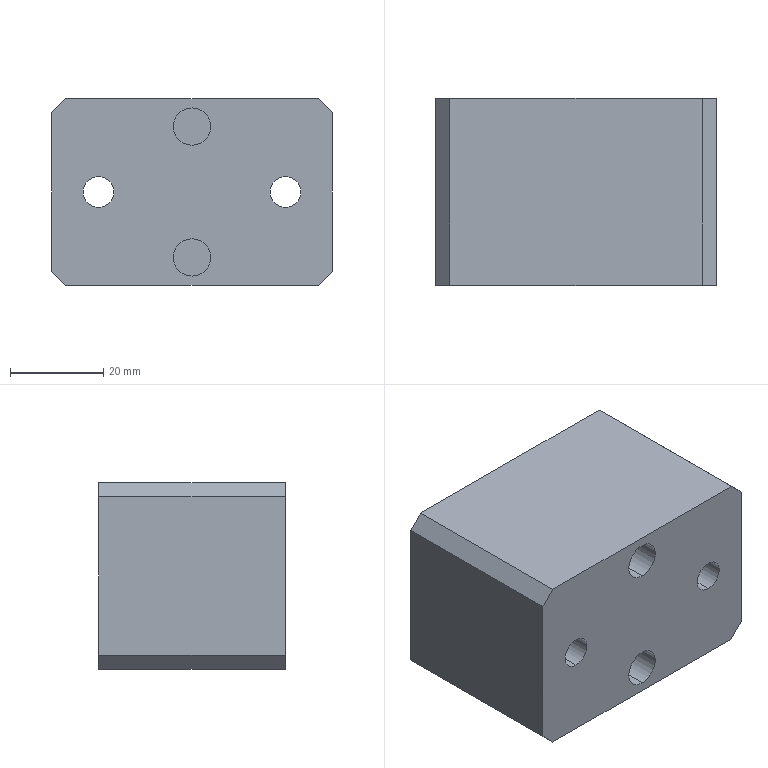Part | SolidWorks | features HoleWzd 4, Chamfer 1, Extrusion 1 | 1 solid | 44 faces | box 60 x 40 x 40 mm | volume 87063 mm3 | cylinder 20 | plane 16 | cone 8 | commonest cylinder face diameters 8 x8 5 x4 6.6 x4 11 x4
STEP:
#1=CARTESIAN_POINT('',(-2.229,-10.711,38.));
#2=VERTEX_POINT('',#1);
#3=CARTESIAN_POINT('',(-2.229,-10.711,30.));
#4=VERTEX_POINT('',#3);
#5=CARTESIAN_POINT('',(-2.229,-10.711,34.));
#6=DIRECTION('',(0.,-1.,0.));
#7=DIRECTION('',(0.,0.,-1.));
#8=AXIS2_PLACEMENT_3D('',#5,#6,#7);
#9=CIRCLE('',#8,4.);
#10=EDGE_CURVE('',#2,#4,#9,.T.);
#11=ORIENTED_EDGE('',*,*,#10,.F.);
#12=CARTESIAN_POINT('',(-2.229,-19.211,38.));
#13=VERTEX_POINT('',#12);
#14=CARTESIAN_POINT('',(-2.229,-19.211,38.));
#15=DIRECTION('',(0.,-1.,0.));
#16=VECTOR('',#15,1000.);
#17=LINE('',#14,#16);
#18=EDGE_CURVE('',#2,#13,#17,.T.);
#19=ORIENTED_EDGE('',*,*,#18,.T.);
#20=CARTESIAN_POINT('',(-2.229,-19.211,30.));
#21=VERTEX_POINT('',#20);
#22=CARTESIAN_POINT('',(-2.229,-19.211,34.));
#23=DIRECTION('',(0.,-1.,0.));
#24=DIRECTION('',(0.,0.,-1.));
#25=AXIS2_PLACEMENT_3D('',#22,#23,#24);
#26=CIRCLE('',#25,4.);
#27=EDGE_CURVE('',#13,#21,#26,.T.);
#28=ORIENTED_EDGE('',*,*,#27,.T.);
#29=CARTESIAN_POINT('',(-2.229,-19.211,30.));
#30=DIRECTION('',(0.,-1.,0.));
#31=VECTOR('',#30,1000.);
#32=LINE('',#29,#31);
#33=EDGE_CURVE('',#4,#21,#32,.T.);
#34=ORIENTED_EDGE('',*,*,#33,.F.);
#35=EDGE_LOOP('',(#11,#19,#28,#34));
#36=FACE_OUTER_BOUND('',#35,.T.);
#37=CARTESIAN_POINT('',(-2.229,-19.211,34.));
#38=DIRECTION('',(0.,-1.,0.));
#39=DIRECTION('',(0.,0.,-1.));
#40=AXIS2_PLACEMENT_3D('',#37,#38,#39);
#41=CYLINDRICAL_SURFACE('',#40,4.);
#42=ADVANCED_FACE('',(#36),#41,.F.);
#43=CARTESIAN_POINT('',(-2.229,-10.711,10.));
#44=VERTEX_POINT('',#43);
#45=CARTESIAN_POINT('',(-2.229,-10.711,2.));
#46=VERTEX_POINT('',#45);
#47=CARTESIAN_POINT('',(-2.229,-10.711,6.));
#48=DIRECTION('',(0.,-1.,0.));
#49=DIRECTION('',(0.,0.,-1.));
#50=AXIS2_PLACEMENT_3D('',#47,#48,#49);
#51=CIRCLE('',#50,4.);
#52=EDGE_CURVE('',#44,#46,#51,.T.);
#53=ORIENTED_EDGE('',*,*,#52,.F.);
#54=CARTESIAN_POINT('',(-2.229,-19.211,10.));
#55=VERTEX_POINT('',#54);
#56=CARTESIAN_POINT('',(-2.229,-19.211,10.));
#57=DIRECTION('',(0.,-1.,0.));
#58=VECTOR('',#57,1000.);
#59=LINE('',#56,#58);
#60=EDGE_CURVE('',#44,#55,#59,.T.);
#61=ORIENTED_EDGE('',*,*,#60,.T.);
#62=CARTESIAN_POINT('',(-2.229,-19.211,2.));
#63=VERTEX_POINT('',#62);
#64=CARTESIAN_POINT('',(-2.229,-19.211,6.));
#65=DIRECTION('',(0.,-1.,0.));
#66=DIRECTION('',(0.,0.,-1.));
#67=AXIS2_PLACEMENT_3D('',#64,#65,#66);
#68=CIRCLE('',#67,4.);
#69=EDGE_CURVE('',#55,#63,#68,.T.);
#70=ORIENTED_EDGE('',*,*,#69,.T.);
#71=CARTESIAN_POINT('',(-2.229,-19.211,2.));
#72=DIRECTION('',(0.,-1.,0.));
#73=VECTOR('',#72,1000.);
#74=LINE('',#71,#73);
#75=EDGE_CURVE('',#46,#63,#74,.T.);
#76=ORIENTED_EDGE('',*,*,#75,.F.);
#77=EDGE_LOOP('',(#53,#61,#70,#76));
#78=FACE_OUTER_BOUND('',#77,.T.);
#79=CARTESIAN_POINT('',(-2.229,-19.211,6.));
#80=DIRECTION('',(0.,-1.,0.));
#81=DIRECTION('',(0.,0.,-1.));
#82=AXIS2_PLACEMENT_3D('',#79,#80,#81);
#83=CYLINDRICAL_SURFACE('',#82,4.);
#84=ADVANCED_FACE('',(#78),#83,.F.);
#85=CARTESIAN_POINT('',(17.771,11.789,4.));
#86=VERTEX_POINT('',#85);
#87=CARTESIAN_POINT('',(17.771,11.789,12.));
#88=VERTEX_POINT('',#87);
#89=CARTESIAN_POINT('',(17.771,11.789,8.));
#90=DIRECTION('',(0.,1.,0.));
#91=DIRECTION('',(0.,0.,1.));
#92=AXIS2_PLACEMENT_3D('',#89,#90,#91);
#93=CIRCLE('',#92,4.);
#94=EDGE_CURVE('',#86,#88,#93,.T.);
#95=ORIENTED_EDGE('',*,*,#94,.F.);
#96=CARTESIAN_POINT('',(17.771,20.789,4.));
#97=VERTEX_POINT('',#96);
#98=CARTESIAN_POINT('',(17.771,20.789,4.));
#99=DIRECTION('',(0.,1.,0.));
#100=VECTOR('',#99,1000.);
#101=LINE('',#98,#100);
#102=EDGE_CURVE('',#86,#97,#101,.T.);
#103=ORIENTED_EDGE('',*,*,#102,.T.);
#104=CARTESIAN_POINT('',(17.771,20.789,12.));
#105=VERTEX_POINT('',#104);
#106=CARTESIAN_POINT('',(17.771,20.789,8.));
#107=DIRECTION('',(0.,1.,0.));
#108=DIRECTION('',(0.,0.,1.));
#109=AXIS2_PLACEMENT_3D('',#106,#107,#108);
#110=CIRCLE('',#109,4.);
#111=EDGE_CURVE('',#97,#105,#110,.T.);
#112=ORIENTED_EDGE('',*,*,#111,.T.);
#113=CARTESIAN_POINT('',(17.771,20.789,12.));
#114=DIRECTION('',(0.,1.,0.));
#115=VECTOR('',#114,1000.);
#116=LINE('',#113,#115);
#117=EDGE_CURVE('',#88,#105,#116,.T.);
#118=ORIENTED_EDGE('',*,*,#117,.F.);
#119=EDGE_LOOP('',(#95,#103,#112,#118));
#120=FACE_OUTER_BOUND('',#119,.T.);
#121=CARTESIAN_POINT('',(17.771,20.789,8.));
#122=DIRECTION('',(0.,1.,0.));
#123=DIRECTION('',(0.,0.,1.));
#124=AXIS2_PLACEMENT_3D('',#121,#122,#123);
#125=CYLINDRICAL_SURFACE('',#124,4.);
#126=ADVANCED_FACE('',(#120),#125,.F.);
#127=CARTESIAN_POINT('',(-22.229,11.789,28.));
#128=VERTEX_POINT('',#127);
#129=CARTESIAN_POINT('',(-22.229,11.789,36.));
#130=VERTEX_POINT('',#129);
#131=CARTESIAN_POINT('',(-22.229,11.789,32.));
#132=DIRECTION('',(0.,1.,0.));
#133=DIRECTION('',(0.,0.,1.));
#134=AXIS2_PLACEMENT_3D('',#131,#132,#133);
#135=CIRCLE('',#134,4.);
#136=EDGE_CURVE('',#128,#130,#135,.T.);
#137=ORIENTED_EDGE('',*,*,#136,.F.);
#138=CARTESIAN_POINT('',(-22.229,20.789,28.));
#139=VERTEX_POINT('',#138);
#140=CARTESIAN_POINT('',(-22.229,20.789,28.));
#141=DIRECTION('',(0.,1.,0.));
#142=VECTOR('',#141,1000.);
#143=LINE('',#140,#142);
#144=EDGE_CURVE('',#128,#139,#143,.T.);
#145=ORIENTED_EDGE('',*,*,#144,.T.);
#146=CARTESIAN_POINT('',(-22.229,20.789,36.));
#147=VERTEX_POINT('',#146);
#148=CARTESIAN_POINT('',(-22.229,20.789,32.));
#149=DIRECTION('',(0.,1.,0.));
#150=DIRECTION('',(0.,0.,1.));
#151=AXIS2_PLACEMENT_3D('',#148,#149,#150);
#152=CIRCLE('',#151,4.);
#153=EDGE_CURVE('',#139,#147,#152,.T.);
#154=ORIENTED_EDGE('',*,*,#153,.T.);
#155=CARTESIAN_POINT('',(-22.229,20.789,36.));
#156=DIRECTION('',(0.,1.,0.));
#157=VECTOR('',#156,1000.);
#158=LINE('',#155,#157);
#159=EDGE_CURVE('',#130,#147,#158,.T.);
#160=ORIENTED_EDGE('',*,*,#159,.F.);
#161=EDGE_LOOP('',(#137,#145,#154,#160));
#162=FACE_OUTER_BOUND('',#161,.T.);
#163=CARTESIAN_POINT('',(-22.229,20.789,32.));
#164=DIRECTION('',(0.,1.,0.));
#165=DIRECTION('',(0.,0.,1.));
#166=AXIS2_PLACEMENT_3D('',#163,#164,#165);
#167=CYLINDRICAL_SURFACE('',#166,4.);
#168=ADVANCED_FACE('',(#162),#167,.F.);
#169=CARTESIAN_POINT('',(-22.229,-6.211,14.5));
#170=VERTEX_POINT('',#169);
#171=CARTESIAN_POINT('',(-22.229,-6.211,25.5));
#172=VERTEX_POINT('',#171);
#173=CARTESIAN_POINT('',(-22.229,-6.211,20.));
#174=DIRECTION('',(0.,1.,0.));
#175=DIRECTION('',(0.,0.,1.));
#176=AXIS2_PLACEMENT_3D('',#173,#174,#175);
#177=CIRCLE('',#176,5.5);
#178=EDGE_CURVE('',#170,#172,#177,.T.);
#179=ORIENTED_EDGE('',*,*,#178,.F.);
#180=CARTESIAN_POINT('',(-22.229,20.789,14.5));
#181=VERTEX_POINT('',#180);
#182=CARTESIAN_POINT('',(-22.229,20.789,14.5));
#183=DIRECTION('',(0.,1.,0.));
#184=VECTOR('',#183,1000.);
#185=LINE('',#182,#184);
#186=EDGE_CURVE('',#170,#181,#185,.T.);
#187=ORIENTED_EDGE('',*,*,#186,.T.);
#188=CARTESIAN_POINT('',(-22.229,20.789,25.5));
#189=VERTEX_POINT('',#188);
#190=CARTESIAN_POINT('',(-22.229,20.789,20.));
#191=DIRECTION('',(0.,1.,0.));
#192=DIRECTION('',(0.,0.,1.));
#193=AXIS2_PLACEMENT_3D('',#190,#191,#192);
#194=CIRCLE('',#193,5.5);
#195=EDGE_CURVE('',#181,#189,#194,.T.);
#196=ORIENTED_EDGE('',*,*,#195,.T.);
#197=CARTESIAN_POINT('',(-22.229,20.789,25.5));
#198=DIRECTION('',(0.,1.,0.));
#199=VECTOR('',#198,1000.);
#200=LINE('',#197,#199);
#201=EDGE_CURVE('',#172,#189,#200,.T.);
#202=ORIENTED_EDGE('',*,*,#201,.F.);
#203=EDGE_LOOP('',(#179,#187,#196,#202));
#204=FACE_OUTER_BOUND('',#203,.T.);
#205=CARTESIAN_POINT('',(-22.229,20.789,20.));
#206=DIRECTION('',(0.,1.,0.));
#207=DIRECTION('',(0.,0.,1.));
#208=AXIS2_PLACEMENT_3D('',#205,#206,#207);
#209=CYLINDRICAL_SURFACE('',#208,5.5);
#210=ADVANCED_FACE('',(#204),#209,.F.);
#211=CARTESIAN_POINT('',(-22.229,-19.211,16.7));
#212=VERTEX_POINT('',#211);
#213=CARTESIAN_POINT('',(-22.229,-19.211,23.3));
#214=VERTEX_POINT('',#213);
#215=CARTESIAN_POINT('',(-22.229,-19.211,20.));
#216=DIRECTION('',(0.,1.,0.));
#217=DIRECTION('',(0.,0.,1.));
#218=AXIS2_PLACEMENT_3D('',#215,#216,#217);
#219=CIRCLE('',#218,3.3);
#220=EDGE_CURVE('',#212,#214,#219,.T.);
#221=ORIENTED_EDGE('',*,*,#220,.F.);
#222=CARTESIAN_POINT('',(-22.229,-6.211,16.7));
#223=VERTEX_POINT('',#222);
#224=CARTESIAN_POINT('',(-22.229,20.789,16.7));
#225=DIRECTION('',(0.,1.,0.));
#226=VECTOR('',#225,1000.);
#227=LINE('',#224,#226);
#228=EDGE_CURVE('',#212,#223,#227,.T.);
#229=ORIENTED_EDGE('',*,*,#228,.T.);
#230=CARTESIAN_POINT('',(-22.229,-6.211,23.3));
#231=VERTEX_POINT('',#230);
#232=CARTESIAN_POINT('',(-22.229,-6.211,20.));
#233=DIRECTION('',(0.,1.,0.));
#234=DIRECTION('',(0.,0.,1.));
#235=AXIS2_PLACEMENT_3D('',#232,#233,#234);
#236=CIRCLE('',#235,3.3);
#237=EDGE_CURVE('',#223,#231,#236,.T.);
#238=ORIENTED_EDGE('',*,*,#237,.T.);
#239=CARTESIAN_POINT('',(-22.229,20.789,23.3));
#240=DIRECTION('',(0.,1.,0.));
#241=VECTOR('',#240,1000.);
#242=LINE('',#239,#241);
#243=EDGE_CURVE('',#214,#231,#242,.T.);
#244=ORIENTED_EDGE('',*,*,#243,.F.);
#245=EDGE_LOOP('',(#221,#229,#238,#244));
#246=FACE_OUTER_BOUND('',#245,.T.);
#247=CARTESIAN_POINT('',(-22.229,20.789,20.));
#248=DIRECTION('',(0.,1.,0.));
#249=DIRECTION('',(0.,0.,1.));
#250=AXIS2_PLACEMENT_3D('',#247,#248,#249);
#251=CYLINDRICAL_SURFACE('',#250,3.3);
#252=ADVANCED_FACE('',(#246),#251,.F.);
#253=CARTESIAN_POINT('',(17.771,-6.211,14.5));
#254=VERTEX_POINT('',#253);
#255=CARTESIAN_POINT('',(17.771,-6.211,25.5));
#256=VERTEX_POINT('',#255);
#257=CARTESIAN_POINT('',(17.771,-6.211,20.));
#258=DIRECTION('',(0.,1.,0.));
#259=DIRECTION('',(0.,0.,1.));
#260=AXIS2_PLACEMENT_3D('',#257,#258,#259);
#261=CIRCLE('',#260,5.5);
#262=EDGE_CURVE('',#254,#256,#261,.T.);
#263=ORIENTED_EDGE('',*,*,#262,.F.);
#264=CARTESIAN_POINT('',(17.771,20.789,14.5));
#265=VERTEX_POINT('',#264);
#266=CARTESIAN_POINT('',(17.771,20.789,14.5));
#267=DIRECTION('',(0.,1.,0.));
#268=VECTOR('',#267,1000.);
#269=LINE('',#266,#268);
#270=EDGE_CURVE('',#254,#265,#269,.T.);
#271=ORIENTED_EDGE('',*,*,#270,.T.);
#272=CARTESIAN_POINT('',(17.771,20.789,25.5));
#273=VERTEX_POINT('',#272);
#274=CARTESIAN_POINT('',(17.771,20.789,20.));
#275=DIRECTION('',(0.,1.,0.));
#276=DIRECTION('',(0.,0.,1.));
#277=AXIS2_PLACEMENT_3D('',#274,#275,#276);
#278=CIRCLE('',#277,5.5);
#279=EDGE_CURVE('',#265,#273,#278,.T.);
#280=ORIENTED_EDGE('',*,*,#279,.T.);
#281=CARTESIAN_POINT('',(17.771,20.789,25.5));
#282=DIRECTION('',(0.,1.,0.));
#283=VECTOR('',#282,1000.);
#284=LINE('',#281,#283);
#285=EDGE_CURVE('',#256,#273,#284,.T.);
#286=ORIENTED_EDGE('',*,*,#285,.F.);
#287=EDGE_LOOP('',(#263,#271,#280,#286));
#288=FACE_OUTER_BOUND('',#287,.T.);
#289=CARTESIAN_POINT('',(17.771,20.789,20.));
#290=DIRECTION('',(0.,1.,0.));
#291=DIRECTION('',(0.,0.,1.));
#292=AXIS2_PLACEMENT_3D('',#289,#290,#291);
#293=CYLINDRICAL_SURFACE('',#292,5.5);
#294=ADVANCED_FACE('',(#288),#293,.F.);
#295=CARTESIAN_POINT('',(17.771,-19.211,16.7));
#296=VERTEX_POINT('',#295);
#297=CARTESIAN_POINT('',(17.771,-19.211,23.3));
#298=VERTEX_POINT('',#297);
#299=CARTESIAN_POINT('',(17.771,-19.211,20.));
#300=DIRECTION('',(0.,1.,0.));
#301=DIRECTION('',(0.,0.,1.));
#302=AXIS2_PLACEMENT_3D('',#299,#300,#301);
#303=CIRCLE('',#302,3.3);
#304=EDGE_CURVE('',#296,#298,#303,.T.);
#305=ORIENTED_EDGE('',*,*,#304,.F.);
#306=CARTESIAN_POINT('',(17.771,-6.211,16.7));
#307=VERTEX_POINT('',#306);
#308=CARTESIAN_POINT('',(17.771,20.789,16.7));
#309=DIRECTION('',(0.,1.,0.));
#310=VECTOR('',#309,1000.);
#311=LINE('',#308,#310);
#312=EDGE_CURVE('',#296,#307,#311,.T.);
#313=ORIENTED_EDGE('',*,*,#312,.T.);
#314=CARTESIAN_POINT('',(17.771,-6.211,23.3));
#315=VERTEX_POINT('',#314);
#316=CARTESIAN_POINT('',(17.771,-6.211,20.));
#317=DIRECTION('',(0.,1.,0.));
#318=DIRECTION('',(0.,0.,1.));
#319=AXIS2_PLACEMENT_3D('',#316,#317,#318);
#320=CIRCLE('',#319,3.3);
#321=EDGE_CURVE('',#307,#315,#320,.T.);
#322=ORIENTED_EDGE('',*,*,#321,.T.);
#323=CARTESIAN_POINT('',(17.771,20.789,23.3));
#324=DIRECTION('',(0.,1.,0.));
#325=VECTOR('',#324,1000.);
#326=LINE('',#323,#325);
#327=EDGE_CURVE('',#298,#315,#326,.T.);
#328=ORIENTED_EDGE('',*,*,#327,.F.);
#329=EDGE_LOOP('',(#305,#313,#322,#328));
#330=FACE_OUTER_BOUND('',#329,.T.);
#331=CARTESIAN_POINT('',(17.771,20.789,20.));
#332=DIRECTION('',(0.,1.,0.));
#333=DIRECTION('',(0.,0.,1.));
#334=AXIS2_PLACEMENT_3D('',#331,#332,#333);
#335=CYLINDRICAL_SURFACE('',#334,3.3);
#336=ADVANCED_FACE('',(#330),#335,.F.);
#337=CARTESIAN_POINT('',(-22.229,20.264,5.5));
#338=VERTEX_POINT('',#337);
#339=CARTESIAN_POINT('',(-22.229,20.264,10.5));
#340=VERTEX_POINT('',#339);
#341=CARTESIAN_POINT('',(-22.229,20.264,8.));
#342=DIRECTION('',(0.,1.,0.));
#343=DIRECTION('',(0.,0.,1.));
#344=AXIS2_PLACEMENT_3D('',#341,#342,#343);
#345=CIRCLE('',#344,2.5);
#346=EDGE_CURVE('',#338,#340,#345,.T.);
#347=ORIENTED_EDGE('',*,*,#346,.F.);
#348=CARTESIAN_POINT('',(-22.229,20.789,4.975));
#349=VERTEX_POINT('',#348);
#350=CARTESIAN_POINT('',(-22.229,20.789,4.975));
#351=DIRECTION('',(0.,0.7071,-0.7071));
#352=VECTOR('',#351,1000.);
#353=LINE('',#350,#352);
#354=EDGE_CURVE('',#338,#349,#353,.T.);
#355=ORIENTED_EDGE('',*,*,#354,.T.);
#356=CARTESIAN_POINT('',(-22.229,20.789,11.025));
#357=VERTEX_POINT('',#356);
#358=CARTESIAN_POINT('',(-22.229,20.789,8.));
#359=DIRECTION('',(0.,1.,0.));
#360=DIRECTION('',(0.,0.,1.));
#361=AXIS2_PLACEMENT_3D('',#358,#359,#360);
#362=CIRCLE('',#361,3.025);
#363=EDGE_CURVE('',#349,#357,#362,.T.);
#364=ORIENTED_EDGE('',*,*,#363,.T.);
#365=CARTESIAN_POINT('',(-22.229,20.789,11.025));
#366=DIRECTION('',(0.,0.7071,0.7071));
#367=VECTOR('',#366,1000.);
#368=LINE('',#365,#367);
#369=EDGE_CURVE('',#340,#357,#368,.T.);
#370=ORIENTED_EDGE('',*,*,#369,.F.);
#371=EDGE_LOOP('',(#347,#355,#364,#370));
#372=FACE_OUTER_BOUND('',#371,.T.);
#373=CARTESIAN_POINT('',(-22.229,20.789,8.));
#374=DIRECTION('',(0.,1.,0.));
#375=DIRECTION('',(0.,0.,1.));
#376=AXIS2_PLACEMENT_3D('',#373,#374,#375);
#377=CONICAL_SURFACE('',#376,3.025,0.7854);
#378=ADVANCED_FACE('',(#372),#377,.F.);
#379=CARTESIAN_POINT('',(-22.229,10.292,5.5));
#380=VERTEX_POINT('',#379);
#381=CARTESIAN_POINT('',(-22.229,10.292,10.5));
#382=VERTEX_POINT('',#381);
#383=CARTESIAN_POINT('',(-22.229,10.292,8.));
#384=DIRECTION('',(0.,1.,0.));
#385=DIRECTION('',(0.,0.,1.));
#386=AXIS2_PLACEMENT_3D('',#383,#384,#385);
#387=CIRCLE('',#386,2.5);
#388=EDGE_CURVE('',#380,#382,#387,.T.);
#389=ORIENTED_EDGE('',*,*,#388,.F.);
#390=CARTESIAN_POINT('',(-22.229,20.789,5.5));
#391=DIRECTION('',(0.,1.,0.));
#392=VECTOR('',#391,1000.);
#393=LINE('',#390,#392);
#394=EDGE_CURVE('',#380,#338,#393,.T.);
#395=ORIENTED_EDGE('',*,*,#394,.T.);
#396=ORIENTED_EDGE('',*,*,#346,.T.);
#397=CARTESIAN_POINT('',(-22.229,20.789,10.5));
#398=DIRECTION('',(0.,1.,0.));
#399=VECTOR('',#398,1000.);
#400=LINE('',#397,#399);
#401=EDGE_CURVE('',#382,#340,#400,.T.);
#402=ORIENTED_EDGE('',*,*,#401,.F.);
#403=EDGE_LOOP('',(#389,#395,#396,#402));
#404=FACE_OUTER_BOUND('',#403,.T.);
#405=CARTESIAN_POINT('',(-22.229,20.789,8.));
#406=DIRECTION('',(0.,1.,0.));
#407=DIRECTION('',(0.,0.,1.));
#408=AXIS2_PLACEMENT_3D('',#405,#406,#407);
#409=CYLINDRICAL_SURFACE('',#408,2.5);
#410=ADVANCED_FACE('',(#404),#409,.F.);
#411=CARTESIAN_POINT('',(-22.229,8.789,8.));
#412=VERTEX_POINT('',#411);
#413=CARTESIAN_POINT('',(-22.229,10.292,10.5));
#414=DIRECTION('',(0.,0.515,0.8572));
#415=VECTOR('',#414,1000.);
#416=LINE('',#413,#415);
#417=EDGE_CURVE('',#412,#382,#416,.T.);
#418=ORIENTED_EDGE('',*,*,#417,.F.);
#419=CARTESIAN_POINT('',(-22.229,10.292,5.5));
#420=DIRECTION('',(0.,0.515,-0.8572));
#421=VECTOR('',#420,1000.);
#422=LINE('',#419,#421);
#423=EDGE_CURVE('',#412,#380,#422,.T.);
#424=ORIENTED_EDGE('',*,*,#423,.T.);
#425=ORIENTED_EDGE('',*,*,#388,.T.);
#426=EDGE_LOOP('',(#418,#424,#425));
#427=FACE_OUTER_BOUND('',#426,.T.);
#428=CARTESIAN_POINT('',(-22.229,10.292,8.));
#429=DIRECTION('',(0.,1.,0.));
#430=DIRECTION('',(0.,0.,1.));
#431=AXIS2_PLACEMENT_3D('',#428,#429,#430);
#432=CONICAL_SURFACE('',#431,2.5,1.03);
#433=ADVANCED_FACE('',(#427),#432,.F.);
#434=CARTESIAN_POINT('',(17.771,20.264,29.5));
#435=VERTEX_POINT('',#434);
#436=CARTESIAN_POINT('',(17.771,20.264,34.5));
#437=VERTEX_POINT('',#436);
#438=CARTESIAN_POINT('',(17.771,20.264,32.));
#439=DIRECTION('',(0.,1.,0.));
#440=DIRECTION('',(0.,0.,1.));
#441=AXIS2_PLACEMENT_3D('',#438,#439,#440);
#442=CIRCLE('',#441,2.5);
#443=EDGE_CURVE('',#435,#437,#442,.T.);
#444=ORIENTED_EDGE('',*,*,#443,.F.);
#445=CARTESIAN_POINT('',(17.771,20.789,28.975));
#446=VERTEX_POINT('',#445);
#447=CARTESIAN_POINT('',(17.771,20.789,28.975));
#448=DIRECTION('',(0.,0.7071,-0.7071));
#449=VECTOR('',#448,1000.);
#450=LINE('',#447,#449);
#451=EDGE_CURVE('',#435,#446,#450,.T.);
#452=ORIENTED_EDGE('',*,*,#451,.T.);
#453=CARTESIAN_POINT('',(17.771,20.789,35.025));
#454=VERTEX_POINT('',#453);
#455=CARTESIAN_POINT('',(17.771,20.789,32.));
#456=DIRECTION('',(0.,1.,0.));
#457=DIRECTION('',(0.,0.,1.));
#458=AXIS2_PLACEMENT_3D('',#455,#456,#457);
#459=CIRCLE('',#458,3.025);
#460=EDGE_CURVE('',#446,#454,#459,.T.);
#461=ORIENTED_EDGE('',*,*,#460,.T.);
#462=CARTESIAN_POINT('',(17.771,20.789,35.025));
#463=DIRECTION('',(0.,0.7071,0.7071));
#464=VECTOR('',#463,1000.);
#465=LINE('',#462,#464);
#466=EDGE_CURVE('',#437,#454,#465,.T.);
#467=ORIENTED_EDGE('',*,*,#466,.F.);
#468=EDGE_LOOP('',(#444,#452,#461,#467));
#469=FACE_OUTER_BOUND('',#468,.T.);
#470=CARTESIAN_POINT('',(17.771,20.789,32.));
#471=DIRECTION('',(0.,1.,0.));
#472=DIRECTION('',(0.,0.,1.));
#473=AXIS2_PLACEMENT_3D('',#470,#471,#472);
#474=CONICAL_SURFACE('',#473,3.025,0.7854);
#475=ADVANCED_FACE('',(#469),#474,.F.);
#476=CARTESIAN_POINT('',(17.771,10.292,29.5));
#477=VERTEX_POINT('',#476);
#478=CARTESIAN_POINT('',(17.771,10.292,34.5));
#479=VERTEX_POINT('',#478);
#480=CARTESIAN_POINT('',(17.771,10.292,32.));
#481=DIRECTION('',(0.,1.,0.));
#482=DIRECTION('',(0.,0.,1.));
#483=AXIS2_PLACEMENT_3D('',#480,#481,#482);
#484=CIRCLE('',#483,2.5);
#485=EDGE_CURVE('',#477,#479,#484,.T.);
#486=ORIENTED_EDGE('',*,*,#485,.F.);
#487=CARTESIAN_POINT('',(17.771,20.789,29.5));
#488=DIRECTION('',(0.,1.,0.));
#489=VECTOR('',#488,1000.);
#490=LINE('',#487,#489);
#491=EDGE_CURVE('',#477,#435,#490,.T.);
#492=ORIENTED_EDGE('',*,*,#491,.T.);
#493=ORIENTED_EDGE('',*,*,#443,.T.);
#494=CARTESIAN_POINT('',(17.771,20.789,34.5));
#495=DIRECTION('',(0.,1.,0.));
#496=VECTOR('',#495,1000.);
#497=LINE('',#494,#496);
#498=EDGE_CURVE('',#479,#437,#497,.T.);
#499=ORIENTED_EDGE('',*,*,#498,.F.);
#500=EDGE_LOOP('',(#486,#492,#493,#499));
#501=FACE_OUTER_BOUND('',#500,.T.);
#502=CARTESIAN_POINT('',(17.771,20.789,32.));
#503=DIRECTION('',(0.,1.,0.));
#504=DIRECTION('',(0.,0.,1.));
#505=AXIS2_PLACEMENT_3D('',#502,#503,#504);
#506=CYLINDRICAL_SURFACE('',#505,2.5);
#507=ADVANCED_FACE('',(#501),#506,.F.);
#508=CARTESIAN_POINT('',(17.771,8.789,32.));
#509=VERTEX_POINT('',#508);
#510=CARTESIAN_POINT('',(17.771,10.292,34.5));
#511=DIRECTION('',(0.,0.515,0.8572));
#512=VECTOR('',#511,1000.);
#513=LINE('',#510,#512);
#514=EDGE_CURVE('',#509,#479,#513,.T.);
#515=ORIENTED_EDGE('',*,*,#514,.F.);
#516=CARTESIAN_POINT('',(17.771,10.292,29.5));
#517=DIRECTION('',(0.,0.515,-0.8572));
#518=VECTOR('',#517,1000.);
#519=LINE('',#516,#518);
#520=EDGE_CURVE('',#509,#477,#519,.T.);
#521=ORIENTED_EDGE('',*,*,#520,.T.);
#522=ORIENTED_EDGE('',*,*,#485,.T.);
#523=EDGE_LOOP('',(#515,#521,#522));
#524=FACE_OUTER_BOUND('',#523,.T.);
#525=CARTESIAN_POINT('',(17.771,10.292,32.));
#526=DIRECTION('',(0.,1.,0.));
#527=DIRECTION('',(0.,0.,1.));
#528=AXIS2_PLACEMENT_3D('',#525,#526,#527);
#529=CONICAL_SURFACE('',#528,2.5,1.03);
#530=ADVANCED_FACE('',(#524),#529,.F.);
#531=CARTESIAN_POINT('',(-32.229,-19.211,37.));
#532=VERTEX_POINT('',#531);
#533=CARTESIAN_POINT('',(-32.229,-19.211,3.));
#534=VERTEX_POINT('',#533);
#535=CARTESIAN_POINT('',(-32.229,-19.211,40.));
#536=DIRECTION('',(0.,0.,-1.));
#537=VECTOR('',#536,1000.);
#538=LINE('',#535,#537);
#539=EDGE_CURVE('',#532,#534,#538,.T.);
#540=ORIENTED_EDGE('',*,*,#539,.F.);
#541=CARTESIAN_POINT('',(-32.229,20.789,37.));
#542=VERTEX_POINT('',#541);
#543=CARTESIAN_POINT('',(-32.229,20.789,37.));
#544=DIRECTION('',(0.,1.,0.));
#545=VECTOR('',#544,1000.);
#546=LINE('',#543,#545);
#547=EDGE_CURVE('',#532,#542,#546,.T.);
#548=ORIENTED_EDGE('',*,*,#547,.T.);
#549=CARTESIAN_POINT('',(-32.229,20.789,3.));
#550=VERTEX_POINT('',#549);
#551=CARTESIAN_POINT('',(-32.229,20.789,40.));
#552=DIRECTION('',(0.,0.,-1.));
#553=VECTOR('',#552,1000.);
#554=LINE('',#551,#553);
#555=EDGE_CURVE('',#542,#550,#554,.T.);
#556=ORIENTED_EDGE('',*,*,#555,.T.);
#557=CARTESIAN_POINT('',(-32.229,20.789,3.));
#558=DIRECTION('',(0.,-1.,0.));
#559=VECTOR('',#558,1000.);
#560=LINE('',#557,#559);
#561=EDGE_CURVE('',#550,#534,#560,.T.);
#562=ORIENTED_EDGE('',*,*,#561,.T.);
#563=EDGE_LOOP('',(#540,#548,#556,#562));
#564=FACE_OUTER_BOUND('',#563,.T.);
#565=CARTESIAN_POINT('',(-32.229,20.789,40.));
#566=DIRECTION('',(1.,0.,0.));
#567=DIRECTION('',(0.,1.,0.));
#568=AXIS2_PLACEMENT_3D('',#565,#566,#567);
#569=PLANE('',#568);
#570=ADVANCED_FACE('',(#564),#569,.F.);
#571=CARTESIAN_POINT('',(-2.229,-19.211,34.));
#572=DIRECTION('',(0.,-1.,0.));
#573=DIRECTION('',(0.,0.,-1.));
#574=AXIS2_PLACEMENT_3D('',#571,#572,#573);
#575=CIRCLE('',#574,4.);
#576=EDGE_CURVE('',#21,#13,#575,.T.);
#577=ORIENTED_EDGE('',*,*,#576,.F.);
#578=ORIENTED_EDGE('',*,*,#27,.F.);
#579=EDGE_LOOP('',(#577,#578));
#580=FACE_BOUND('',#579,.T.);
#581=CARTESIAN_POINT('',(-2.229,-19.211,6.));
#582=DIRECTION('',(0.,-1.,0.));
#583=DIRECTION('',(0.,0.,-1.));
#584=AXIS2_PLACEMENT_3D('',#581,#582,#583);
#585=CIRCLE('',#584,4.);
#586=EDGE_CURVE('',#63,#55,#585,.T.);
#587=ORIENTED_EDGE('',*,*,#586,.F.);
#588=ORIENTED_EDGE('',*,*,#69,.F.);
#589=EDGE_LOOP('',(#587,#588));
#590=FACE_BOUND('',#589,.T.);
#591=CARTESIAN_POINT('',(-22.229,-19.211,20.));
#592=DIRECTION('',(0.,1.,0.));
#593=DIRECTION('',(0.,0.,1.));
#594=AXIS2_PLACEMENT_3D('',#591,#592,#593);
#595=CIRCLE('',#594,3.3);
#596=EDGE_CURVE('',#214,#212,#595,.T.);
#597=ORIENTED_EDGE('',*,*,#596,.T.);
#598=ORIENTED_EDGE('',*,*,#220,.T.);
#599=EDGE_LOOP('',(#597,#598));
#600=FACE_BOUND('',#599,.T.);
#601=CARTESIAN_POINT('',(17.771,-19.211,20.));
#602=DIRECTION('',(0.,1.,0.));
#603=DIRECTION('',(0.,0.,1.));
#604=AXIS2_PLACEMENT_3D('',#601,#602,#603);
#605=CIRCLE('',#604,3.3);
#606=EDGE_CURVE('',#298,#296,#605,.T.);
#607=ORIENTED_EDGE('',*,*,#606,.T.);
#608=ORIENTED_EDGE('',*,*,#304,.T.);
#609=EDGE_LOOP('',(#607,#608));
#610=FACE_BOUND('',#609,.T.);
#611=CARTESIAN_POINT('',(27.771,-19.211,37.));
#612=VERTEX_POINT('',#611);
#613=CARTESIAN_POINT('',(27.771,-19.211,3.));
#614=VERTEX_POINT('',#613);
#615=CARTESIAN_POINT('',(27.771,-19.211,40.));
#616=DIRECTION('',(0.,0.,-1.));
#617=VECTOR('',#616,1000.);
#618=LINE('',#615,#617);
#619=EDGE_CURVE('',#612,#614,#618,.T.);
#620=ORIENTED_EDGE('',*,*,#619,.F.);
#621=CARTESIAN_POINT('',(24.771,-19.211,40.));
#622=VERTEX_POINT('',#621);
#623=CARTESIAN_POINT('',(24.771,-19.211,40.));
#624=DIRECTION('',(-0.7071,0.,0.7071));
#625=VECTOR('',#624,1000.);
#626=LINE('',#623,#625);
#627=EDGE_CURVE('',#612,#622,#626,.T.);
#628=ORIENTED_EDGE('',*,*,#627,.T.);
#629=CARTESIAN_POINT('',(-29.229,-19.211,40.));
#630=VERTEX_POINT('',#629);
#631=CARTESIAN_POINT('',(-32.229,-19.211,40.));
#632=DIRECTION('',(1.,0.,0.));
#633=VECTOR('',#632,1000.);
#634=LINE('',#631,#633);
#635=EDGE_CURVE('',#630,#622,#634,.T.);
#636=ORIENTED_EDGE('',*,*,#635,.F.);
#637=CARTESIAN_POINT('',(-29.229,-19.211,40.));
#638=DIRECTION('',(-0.7071,0.,-0.7071));
#639=VECTOR('',#638,1000.);
#640=LINE('',#637,#639);
#641=EDGE_CURVE('',#630,#532,#640,.T.);
#642=ORIENTED_EDGE('',*,*,#641,.T.);
#643=ORIENTED_EDGE('',*,*,#539,.T.);
#644=CARTESIAN_POINT('',(-29.229,-19.211,0.));
#645=VERTEX_POINT('',#644);
#646=CARTESIAN_POINT('',(-32.229,-19.211,3.));
#647=DIRECTION('',(0.7071,0.,-0.7071));
#648=VECTOR('',#647,1000.);
#649=LINE('',#646,#648);
#650=EDGE_CURVE('',#534,#645,#649,.T.);
#651=ORIENTED_EDGE('',*,*,#650,.T.);
#652=CARTESIAN_POINT('',(24.771,-19.211,0.));
#653=VERTEX_POINT('',#652);
#654=CARTESIAN_POINT('',(-32.229,-19.211,0.));
#655=DIRECTION('',(1.,0.,0.));
#656=VECTOR('',#655,1000.);
#657=LINE('',#654,#656);
#658=EDGE_CURVE('',#645,#653,#657,.T.);
#659=ORIENTED_EDGE('',*,*,#658,.T.);
#660=CARTESIAN_POINT('',(27.771,-19.211,3.));
#661=DIRECTION('',(0.7071,0.,0.7071));
#662=VECTOR('',#661,1000.);
#663=LINE('',#660,#662);
#664=EDGE_CURVE('',#653,#614,#663,.T.);
#665=ORIENTED_EDGE('',*,*,#664,.T.);
#666=EDGE_LOOP('',(#620,#628,#636,#642,#643,#651,#659,#665));
#667=FACE_OUTER_BOUND('',#666,.T.);
#668=CARTESIAN_POINT('',(-32.229,-19.211,40.));
#669=DIRECTION('',(0.,1.,0.));
#670=DIRECTION('',(0.,0.,1.));
#671=AXIS2_PLACEMENT_3D('',#668,#669,#670);
#672=PLANE('',#671);
#673=ADVANCED_FACE('',(#580,#590,#600,#610,#667),#672,.F.);
#674=CARTESIAN_POINT('',(27.771,20.789,37.));
#675=VERTEX_POINT('',#674);
#676=CARTESIAN_POINT('',(27.771,20.789,3.));
#677=VERTEX_POINT('',#676);
#678=CARTESIAN_POINT('',(27.771,20.789,40.));
#679=DIRECTION('',(0.,0.,-1.));
#680=VECTOR('',#679,1000.);
#681=LINE('',#678,#680);
#682=EDGE_CURVE('',#675,#677,#681,.T.);
#683=ORIENTED_EDGE('',*,*,#682,.F.);
#684=CARTESIAN_POINT('',(27.771,-19.211,37.));
#685=DIRECTION('',(0.,-1.,0.));
#686=VECTOR('',#685,1000.);
#687=LINE('',#684,#686);
#688=EDGE_CURVE('',#675,#612,#687,.T.);
#689=ORIENTED_EDGE('',*,*,#688,.T.);
#690=ORIENTED_EDGE('',*,*,#619,.T.);
#691=CARTESIAN_POINT('',(27.771,20.789,3.));
#692=DIRECTION('',(0.,1.,0.));
#693=VECTOR('',#692,1000.);
#694=LINE('',#691,#693);
#695=EDGE_CURVE('',#614,#677,#694,.T.);
#696=ORIENTED_EDGE('',*,*,#695,.T.);
#697=EDGE_LOOP('',(#683,#689,#690,#696));
#698=FACE_OUTER_BOUND('',#697,.T.);
#699=CARTESIAN_POINT('',(27.771,20.789,40.));
#700=DIRECTION('',(-1.,0.,0.));
#701=DIRECTION('',(0.,-1.,0.));
#702=AXIS2_PLACEMENT_3D('',#699,#700,#701);
#703=PLANE('',#702);
#704=ADVANCED_FACE('',(#698),#703,.F.);
#705=CARTESIAN_POINT('',(17.771,20.789,8.));
#706=DIRECTION('',(0.,1.,0.));
#707=DIRECTION('',(0.,0.,1.));
#708=AXIS2_PLACEMENT_3D('',#705,#706,#707);
#709=CIRCLE('',#708,4.);
#710=EDGE_CURVE('',#105,#97,#709,.T.);
#711=ORIENTED_EDGE('',*,*,#710,.F.);
#712=ORIENTED_EDGE('',*,*,#111,.F.);
#713=EDGE_LOOP('',(#711,#712));
#714=FACE_BOUND('',#713,.T.);
#715=CARTESIAN_POINT('',(-22.229,20.789,32.));
#716=DIRECTION('',(0.,1.,0.));
#717=DIRECTION('',(0.,0.,1.));
#718=AXIS2_PLACEMENT_3D('',#715,#716,#717);
#719=CIRCLE('',#718,4.);
#720=EDGE_CURVE('',#147,#139,#719,.T.);
#721=ORIENTED_EDGE('',*,*,#720,.F.);
#722=ORIENTED_EDGE('',*,*,#153,.F.);
#723=EDGE_LOOP('',(#721,#722));
#724=FACE_BOUND('',#723,.T.);
#725=CARTESIAN_POINT('',(-22.229,20.789,20.));
#726=DIRECTION('',(0.,1.,0.));
#727=DIRECTION('',(0.,0.,1.));
#728=AXIS2_PLACEMENT_3D('',#725,#726,#727);
#729=CIRCLE('',#728,5.5);
#730=EDGE_CURVE('',#189,#181,#729,.T.);
#731=ORIENTED_EDGE('',*,*,#730,.F.);
#732=ORIENTED_EDGE('',*,*,#195,.F.);
#733=EDGE_LOOP('',(#731,#732));
#734=FACE_BOUND('',#733,.T.);
#735=CARTESIAN_POINT('',(17.771,20.789,20.));
#736=DIRECTION('',(0.,1.,0.));
#737=DIRECTION('',(0.,0.,1.));
#738=AXIS2_PLACEMENT_3D('',#735,#736,#737);
#739=CIRCLE('',#738,5.5);
#740=EDGE_CURVE('',#273,#265,#739,.T.);
#741=ORIENTED_EDGE('',*,*,#740,.F.);
#742=ORIENTED_EDGE('',*,*,#279,.F.);
#743=EDGE_LOOP('',(#741,#742));
#744=FACE_BOUND('',#743,.T.);
#745=CARTESIAN_POINT('',(-22.229,20.789,8.));
#746=DIRECTION('',(0.,1.,0.));
#747=DIRECTION('',(0.,0.,1.));
#748=AXIS2_PLACEMENT_3D('',#745,#746,#747);
#749=CIRCLE('',#748,3.025);
#750=EDGE_CURVE('',#357,#349,#749,.T.);
#751=ORIENTED_EDGE('',*,*,#750,.F.);
#752=ORIENTED_EDGE('',*,*,#363,.F.);
#753=EDGE_LOOP('',(#751,#752));
#754=FACE_BOUND('',#753,.T.);
#755=CARTESIAN_POINT('',(17.771,20.789,32.));
#756=DIRECTION('',(0.,1.,0.));
#757=DIRECTION('',(0.,0.,1.));
#758=AXIS2_PLACEMENT_3D('',#755,#756,#757);
#759=CIRCLE('',#758,3.025);
#760=EDGE_CURVE('',#454,#446,#759,.T.);
#761=ORIENTED_EDGE('',*,*,#760,.F.);
#762=ORIENTED_EDGE('',*,*,#460,.F.);
#763=EDGE_LOOP('',(#761,#762));
#764=FACE_BOUND('',#763,.T.);
#765=CARTESIAN_POINT('',(24.771,20.789,40.));
#766=VERTEX_POINT('',#765);
#767=CARTESIAN_POINT('',(-29.229,20.789,40.));
#768=VERTEX_POINT('',#767);
#769=CARTESIAN_POINT('',(-32.229,20.789,40.));
#770=DIRECTION('',(-1.,0.,0.));
#771=VECTOR('',#770,1000.);
#772=LINE('',#769,#771);
#773=EDGE_CURVE('',#766,#768,#772,.T.);
#774=ORIENTED_EDGE('',*,*,#773,.F.);
#775=CARTESIAN_POINT('',(24.771,20.789,40.));
#776=DIRECTION('',(0.7071,0.,-0.7071));
#777=VECTOR('',#776,1000.);
#778=LINE('',#775,#777);
#779=EDGE_CURVE('',#766,#675,#778,.T.);
#780=ORIENTED_EDGE('',*,*,#779,.T.);
#781=ORIENTED_EDGE('',*,*,#682,.T.);
#782=CARTESIAN_POINT('',(24.771,20.789,0.));
#783=VERTEX_POINT('',#782);
#784=CARTESIAN_POINT('',(27.771,20.789,3.));
#785=DIRECTION('',(-0.7071,0.,-0.7071));
#786=VECTOR('',#785,1000.);
#787=LINE('',#784,#786);
#788=EDGE_CURVE('',#677,#783,#787,.T.);
#789=ORIENTED_EDGE('',*,*,#788,.T.);
#790=CARTESIAN_POINT('',(-29.229,20.789,0.));
#791=VERTEX_POINT('',#790);
#792=CARTESIAN_POINT('',(-32.229,20.789,0.));
#793=DIRECTION('',(-1.,0.,0.));
#794=VECTOR('',#793,1000.);
#795=LINE('',#792,#794);
#796=EDGE_CURVE('',#783,#791,#795,.T.);
#797=ORIENTED_EDGE('',*,*,#796,.T.);
#798=CARTESIAN_POINT('',(-32.229,20.789,3.));
#799=DIRECTION('',(-0.7071,0.,0.7071));
#800=VECTOR('',#799,1000.);
#801=LINE('',#798,#800);
#802=EDGE_CURVE('',#791,#550,#801,.T.);
#803=ORIENTED_EDGE('',*,*,#802,.T.);
#804=ORIENTED_EDGE('',*,*,#555,.F.);
#805=CARTESIAN_POINT('',(-29.229,20.789,40.));
#806=DIRECTION('',(0.7071,0.,0.7071));
#807=VECTOR('',#806,1000.);
#808=LINE('',#805,#807);
#809=EDGE_CURVE('',#542,#768,#808,.T.);
#810=ORIENTED_EDGE('',*,*,#809,.T.);
#811=EDGE_LOOP('',(#774,#780,#781,#789,#797,#803,#804,#810));
#812=FACE_OUTER_BOUND('',#811,.T.);
#813=CARTESIAN_POINT('',(-32.229,20.789,40.));
#814=DIRECTION('',(0.,-1.,0.));
#815=DIRECTION('',(0.,0.,-1.));
#816=AXIS2_PLACEMENT_3D('',#813,#814,#815);
#817=PLANE('',#816);
#818=ADVANCED_FACE('',(#714,#724,#734,#744,#754,#764,#812),#817,.F.);
#819=ORIENTED_EDGE('',*,*,#635,.T.);
#820=CARTESIAN_POINT('',(24.771,20.789,40.));
#821=DIRECTION('',(0.,1.,0.));
#822=VECTOR('',#821,1000.);
#823=LINE('',#820,#822);
#824=EDGE_CURVE('',#622,#766,#823,.T.);
#825=ORIENTED_EDGE('',*,*,#824,.T.);
#826=ORIENTED_EDGE('',*,*,#773,.T.);
#827=CARTESIAN_POINT('',(-29.229,-19.211,40.));
#828=DIRECTION('',(0.,-1.,0.));
#829=VECTOR('',#828,1000.);
#830=LINE('',#827,#829);
#831=EDGE_CURVE('',#768,#630,#830,.T.);
#832=ORIENTED_EDGE('',*,*,#831,.T.);
#833=EDGE_LOOP('',(#819,#825,#826,#832));
#834=FACE_OUTER_BOUND('',#833,.T.);
#835=CARTESIAN_POINT('',(0.,0.,40.));
#836=DIRECTION('',(0.,0.,1.));
#837=DIRECTION('',(1.,0.,0.));
#838=AXIS2_PLACEMENT_3D('',#835,#836,#837);
#839=PLANE('',#838);
#840=ADVANCED_FACE('',(#834),#839,.T.);
#841=ORIENTED_EDGE('',*,*,#796,.F.);
#842=CARTESIAN_POINT('',(24.771,0.,0.));
#843=DIRECTION('',(0.,-1.,0.));
#844=VECTOR('',#843,1000.);
#845=LINE('',#842,#844);
#846=EDGE_CURVE('',#783,#653,#845,.T.);
#847=ORIENTED_EDGE('',*,*,#846,.T.);
#848=ORIENTED_EDGE('',*,*,#658,.F.);
#849=CARTESIAN_POINT('',(-29.229,0.,0.));
#850=DIRECTION('',(0.,1.,0.));
#851=VECTOR('',#850,1000.);
#852=LINE('',#849,#851);
#853=EDGE_CURVE('',#645,#791,#852,.T.);
#854=ORIENTED_EDGE('',*,*,#853,.T.);
#855=EDGE_LOOP('',(#841,#847,#848,#854));
#856=FACE_OUTER_BOUND('',#855,.T.);
#857=CARTESIAN_POINT('',(0.,0.,0.));
#858=DIRECTION('',(0.,0.,1.));
#859=DIRECTION('',(1.,0.,0.));
#860=AXIS2_PLACEMENT_3D('',#857,#858,#859);
#861=PLANE('',#860);
#862=ADVANCED_FACE('',(#856),#861,.F.);
#863=ORIENTED_EDGE('',*,*,#627,.F.);
#864=ORIENTED_EDGE('',*,*,#688,.F.);
#865=ORIENTED_EDGE('',*,*,#779,.F.);
#866=ORIENTED_EDGE('',*,*,#824,.F.);
#867=EDGE_LOOP('',(#863,#864,#865,#866));
#868=FACE_OUTER_BOUND('',#867,.T.);
#869=CARTESIAN_POINT('',(24.771,0.,40.));
#870=DIRECTION('',(0.7071,0.,0.7071));
#871=DIRECTION('',(0.,-1.,0.));
#872=AXIS2_PLACEMENT_3D('',#869,#870,#871);
#873=PLANE('',#872);
#874=ADVANCED_FACE('',(#868),#873,.T.);
#875=ORIENTED_EDGE('',*,*,#664,.F.);
#876=ORIENTED_EDGE('',*,*,#846,.F.);
#877=ORIENTED_EDGE('',*,*,#788,.F.);
#878=ORIENTED_EDGE('',*,*,#695,.F.);
#879=EDGE_LOOP('',(#875,#876,#877,#878));
#880=FACE_OUTER_BOUND('',#879,.T.);
#881=CARTESIAN_POINT('',(27.771,20.789,3.));
#882=DIRECTION('',(-0.7071,0.,0.7071));
#883=DIRECTION('',(0.,1.,0.));
#884=AXIS2_PLACEMENT_3D('',#881,#882,#883);
#885=PLANE('',#884);
#886=ADVANCED_FACE('',(#880),#885,.F.);
#887=ORIENTED_EDGE('',*,*,#809,.F.);
#888=ORIENTED_EDGE('',*,*,#547,.F.);
#889=ORIENTED_EDGE('',*,*,#641,.F.);
#890=ORIENTED_EDGE('',*,*,#831,.F.);
#891=EDGE_LOOP('',(#887,#888,#889,#890));
#892=FACE_OUTER_BOUND('',#891,.T.);
#893=CARTESIAN_POINT('',(-29.229,0.,40.));
#894=DIRECTION('',(-0.7071,0.,0.7071));
#895=DIRECTION('',(0.,1.,0.));
#896=AXIS2_PLACEMENT_3D('',#893,#894,#895);
#897=PLANE('',#896);
#898=ADVANCED_FACE('',(#892),#897,.T.);
#899=ORIENTED_EDGE('',*,*,#802,.F.);
#900=ORIENTED_EDGE('',*,*,#853,.F.);
#901=ORIENTED_EDGE('',*,*,#650,.F.);
#902=ORIENTED_EDGE('',*,*,#561,.F.);
#903=EDGE_LOOP('',(#899,#900,#901,#902));
#904=FACE_OUTER_BOUND('',#903,.T.);
#905=CARTESIAN_POINT('',(-32.229,20.789,3.));
#906=DIRECTION('',(0.7071,0.,0.7071));
#907=DIRECTION('',(0.,-1.,0.));
#908=AXIS2_PLACEMENT_3D('',#905,#906,#907);
#909=PLANE('',#908);
#910=ADVANCED_FACE('',(#904),#909,.F.);
#911=ORIENTED_EDGE('',*,*,#520,.F.);
#912=ORIENTED_EDGE('',*,*,#514,.T.);
#913=CARTESIAN_POINT('',(17.771,10.292,32.));
#914=DIRECTION('',(0.,1.,0.));
#915=DIRECTION('',(0.,0.,1.));
#916=AXIS2_PLACEMENT_3D('',#913,#914,#915);
#917=CIRCLE('',#916,2.5);
#918=EDGE_CURVE('',#479,#477,#917,.T.);
#919=ORIENTED_EDGE('',*,*,#918,.T.);
#920=EDGE_LOOP('',(#911,#912,#919));
#921=FACE_OUTER_BOUND('',#920,.T.);
#922=CARTESIAN_POINT('',(17.771,10.292,32.));
#923=DIRECTION('',(0.,1.,0.));
#924=DIRECTION('',(0.,0.,1.));
#925=AXIS2_PLACEMENT_3D('',#922,#923,#924);
#926=CONICAL_SURFACE('',#925,2.5,1.03);
#927=ADVANCED_FACE('',(#921),#926,.F.);
#928=ORIENTED_EDGE('',*,*,#491,.F.);
#929=ORIENTED_EDGE('',*,*,#918,.F.);
#930=ORIENTED_EDGE('',*,*,#498,.T.);
#931=CARTESIAN_POINT('',(17.771,20.264,32.));
#932=DIRECTION('',(0.,1.,0.));
#933=DIRECTION('',(0.,0.,1.));
#934=AXIS2_PLACEMENT_3D('',#931,#932,#933);
#935=CIRCLE('',#934,2.5);
#936=EDGE_CURVE('',#437,#435,#935,.T.);
#937=ORIENTED_EDGE('',*,*,#936,.T.);
#938=EDGE_LOOP('',(#928,#929,#930,#937));
#939=FACE_OUTER_BOUND('',#938,.T.);
#940=CARTESIAN_POINT('',(17.771,20.789,32.));
#941=DIRECTION('',(0.,1.,0.));
#942=DIRECTION('',(0.,0.,1.));
#943=AXIS2_PLACEMENT_3D('',#940,#941,#942);
#944=CYLINDRICAL_SURFACE('',#943,2.5);
#945=ADVANCED_FACE('',(#939),#944,.F.);
#946=ORIENTED_EDGE('',*,*,#451,.F.);
#947=ORIENTED_EDGE('',*,*,#936,.F.);
#948=ORIENTED_EDGE('',*,*,#466,.T.);
#949=ORIENTED_EDGE('',*,*,#760,.T.);
#950=EDGE_LOOP('',(#946,#947,#948,#949));
#951=FACE_OUTER_BOUND('',#950,.T.);
#952=CARTESIAN_POINT('',(17.771,20.789,32.));
#953=DIRECTION('',(0.,1.,0.));
#954=DIRECTION('',(0.,0.,1.));
#955=AXIS2_PLACEMENT_3D('',#952,#953,#954);
#956=CONICAL_SURFACE('',#955,3.025,0.7854);
#957=ADVANCED_FACE('',(#951),#956,.F.);
#958=ORIENTED_EDGE('',*,*,#423,.F.);
#959=ORIENTED_EDGE('',*,*,#417,.T.);
#960=CARTESIAN_POINT('',(-22.229,10.292,8.));
#961=DIRECTION('',(0.,1.,0.));
#962=DIRECTION('',(0.,0.,1.));
#963=AXIS2_PLACEMENT_3D('',#960,#961,#962);
#964=CIRCLE('',#963,2.5);
#965=EDGE_CURVE('',#382,#380,#964,.T.);
#966=ORIENTED_EDGE('',*,*,#965,.T.);
#967=EDGE_LOOP('',(#958,#959,#966));
#968=FACE_OUTER_BOUND('',#967,.T.);
#969=CARTESIAN_POINT('',(-22.229,10.292,8.));
#970=DIRECTION('',(0.,1.,0.));
#971=DIRECTION('',(0.,0.,1.));
#972=AXIS2_PLACEMENT_3D('',#969,#970,#971);
#973=CONICAL_SURFACE('',#972,2.5,1.03);
#974=ADVANCED_FACE('',(#968),#973,.F.);
#975=ORIENTED_EDGE('',*,*,#394,.F.);
#976=ORIENTED_EDGE('',*,*,#965,.F.);
#977=ORIENTED_EDGE('',*,*,#401,.T.);
#978=CARTESIAN_POINT('',(-22.229,20.264,8.));
#979=DIRECTION('',(0.,1.,0.));
#980=DIRECTION('',(0.,0.,1.));
#981=AXIS2_PLACEMENT_3D('',#978,#979,#980);
#982=CIRCLE('',#981,2.5);
#983=EDGE_CURVE('',#340,#338,#982,.T.);
#984=ORIENTED_EDGE('',*,*,#983,.T.);
#985=EDGE_LOOP('',(#975,#976,#977,#984));
#986=FACE_OUTER_BOUND('',#985,.T.);
#987=CARTESIAN_POINT('',(-22.229,20.789,8.));
#988=DIRECTION('',(0.,1.,0.));
#989=DIRECTION('',(0.,0.,1.));
#990=AXIS2_PLACEMENT_3D('',#987,#988,#989);
#991=CYLINDRICAL_SURFACE('',#990,2.5);
#992=ADVANCED_FACE('',(#986),#991,.F.);
#993=ORIENTED_EDGE('',*,*,#354,.F.);
#994=ORIENTED_EDGE('',*,*,#983,.F.);
#995=ORIENTED_EDGE('',*,*,#369,.T.);
#996=ORIENTED_EDGE('',*,*,#750,.T.);
#997=EDGE_LOOP('',(#993,#994,#995,#996));
#998=FACE_OUTER_BOUND('',#997,.T.);
#999=CARTESIAN_POINT('',(-22.229,20.789,8.));
#1000=DIRECTION('',(0.,1.,0.));
#1001=DIRECTION('',(0.,0.,1.));
#1002=AXIS2_PLACEMENT_3D('',#999,#1000,#1001);
#1003=CONICAL_SURFACE('',#1002,3.025,0.7854);
#1004=ADVANCED_FACE('',(#998),#1003,.F.);
#1005=ORIENTED_EDGE('',*,*,#312,.F.);
#1006=ORIENTED_EDGE('',*,*,#606,.F.);
#1007=ORIENTED_EDGE('',*,*,#327,.T.);
#1008=CARTESIAN_POINT('',(17.771,-6.211,20.));
#1009=DIRECTION('',(0.,1.,0.));
#1010=DIRECTION('',(0.,0.,1.));
#1011=AXIS2_PLACEMENT_3D('',#1008,#1009,#1010);
#1012=CIRCLE('',#1011,3.3);
#1013=EDGE_CURVE('',#315,#307,#1012,.T.);
#1014=ORIENTED_EDGE('',*,*,#1013,.T.);
#1015=EDGE_LOOP('',(#1005,#1006,#1007,#1014));
#1016=FACE_OUTER_BOUND('',#1015,.T.);
#1017=CARTESIAN_POINT('',(17.771,20.789,20.));
#1018=DIRECTION('',(0.,1.,0.));
#1019=DIRECTION('',(0.,0.,1.));
#1020=AXIS2_PLACEMENT_3D('',#1017,#1018,#1019);
#1021=CYLINDRICAL_SURFACE('',#1020,3.3);
#1022=ADVANCED_FACE('',(#1016),#1021,.F.);
#1023=ORIENTED_EDGE('',*,*,#1013,.F.);
#1024=ORIENTED_EDGE('',*,*,#321,.F.);
#1025=EDGE_LOOP('',(#1023,#1024));
#1026=FACE_BOUND('',#1025,.T.);
#1027=CARTESIAN_POINT('',(17.771,-6.211,20.));
#1028=DIRECTION('',(0.,1.,0.));
#1029=DIRECTION('',(0.,0.,1.));
#1030=AXIS2_PLACEMENT_3D('',#1027,#1028,#1029);
#1031=CIRCLE('',#1030,5.5);
#1032=EDGE_CURVE('',#256,#254,#1031,.T.);
#1033=ORIENTED_EDGE('',*,*,#1032,.T.);
#1034=ORIENTED_EDGE('',*,*,#262,.T.);
#1035=EDGE_LOOP('',(#1033,#1034));
#1036=FACE_OUTER_BOUND('',#1035,.T.);
#1037=CARTESIAN_POINT('',(21.071,-6.211,20.));
#1038=DIRECTION('',(0.,-1.,0.));
#1039=DIRECTION('',(0.,0.,-1.));
#1040=AXIS2_PLACEMENT_3D('',#1037,#1038,#1039);
#1041=PLANE('',#1040);
#1042=ADVANCED_FACE('',(#1026,#1036),#1041,.F.);
#1043=ORIENTED_EDGE('',*,*,#270,.F.);
#1044=ORIENTED_EDGE('',*,*,#1032,.F.);
#1045=ORIENTED_EDGE('',*,*,#285,.T.);
#1046=ORIENTED_EDGE('',*,*,#740,.T.);
#1047=EDGE_LOOP('',(#1043,#1044,#1045,#1046));
#1048=FACE_OUTER_BOUND('',#1047,.T.);
#1049=CARTESIAN_POINT('',(17.771,20.789,20.));
#1050=DIRECTION('',(0.,1.,0.));
#1051=DIRECTION('',(0.,0.,1.));
#1052=AXIS2_PLACEMENT_3D('',#1049,#1050,#1051);
#1053=CYLINDRICAL_SURFACE('',#1052,5.5);
#1054=ADVANCED_FACE('',(#1048),#1053,.F.);
#1055=ORIENTED_EDGE('',*,*,#228,.F.);
#1056=ORIENTED_EDGE('',*,*,#596,.F.);
#1057=ORIENTED_EDGE('',*,*,#243,.T.);
#1058=CARTESIAN_POINT('',(-22.229,-6.211,20.));
#1059=DIRECTION('',(0.,1.,0.));
#1060=DIRECTION('',(0.,0.,1.));
#1061=AXIS2_PLACEMENT_3D('',#1058,#1059,#1060);
#1062=CIRCLE('',#1061,3.3);
#1063=EDGE_CURVE('',#231,#223,#1062,.T.);
#1064=ORIENTED_EDGE('',*,*,#1063,.T.);
#1065=EDGE_LOOP('',(#1055,#1056,#1057,#1064));
#1066=FACE_OUTER_BOUND('',#1065,.T.);
#1067=CARTESIAN_POINT('',(-22.229,20.789,20.));
#1068=DIRECTION('',(0.,1.,0.));
#1069=DIRECTION('',(0.,0.,1.));
#1070=AXIS2_PLACEMENT_3D('',#1067,#1068,#1069);
#1071=CYLINDRICAL_SURFACE('',#1070,3.3);
#1072=ADVANCED_FACE('',(#1066),#1071,.F.);
#1073=ORIENTED_EDGE('',*,*,#1063,.F.);
#1074=ORIENTED_EDGE('',*,*,#237,.F.);
#1075=EDGE_LOOP('',(#1073,#1074));
#1076=FACE_BOUND('',#1075,.T.);
#1077=CARTESIAN_POINT('',(-22.229,-6.211,20.));
#1078=DIRECTION('',(0.,1.,0.));
#1079=DIRECTION('',(0.,0.,1.));
#1080=AXIS2_PLACEMENT_3D('',#1077,#1078,#1079);
#1081=CIRCLE('',#1080,5.5);
#1082=EDGE_CURVE('',#172,#170,#1081,.T.);
#1083=ORIENTED_EDGE('',*,*,#1082,.T.);
#1084=ORIENTED_EDGE('',*,*,#178,.T.);
#1085=EDGE_LOOP('',(#1083,#1084));
#1086=FACE_OUTER_BOUND('',#1085,.T.);
#1087=CARTESIAN_POINT('',(-18.929,-6.211,20.));
#1088=DIRECTION('',(0.,-1.,0.));
#1089=DIRECTION('',(0.,0.,-1.));
#1090=AXIS2_PLACEMENT_3D('',#1087,#1088,#1089);
#1091=PLANE('',#1090);
#1092=ADVANCED_FACE('',(#1076,#1086),#1091,.F.);
#1093=ORIENTED_EDGE('',*,*,#186,.F.);
#1094=ORIENTED_EDGE('',*,*,#1082,.F.);
#1095=ORIENTED_EDGE('',*,*,#201,.T.);
#1096=ORIENTED_EDGE('',*,*,#730,.T.);
#1097=EDGE_LOOP('',(#1093,#1094,#1095,#1096));
#1098=FACE_OUTER_BOUND('',#1097,.T.);
#1099=CARTESIAN_POINT('',(-22.229,20.789,20.));
#1100=DIRECTION('',(0.,1.,0.));
#1101=DIRECTION('',(0.,0.,1.));
#1102=AXIS2_PLACEMENT_3D('',#1099,#1100,#1101);
#1103=CYLINDRICAL_SURFACE('',#1102,5.5);
#1104=ADVANCED_FACE('',(#1098),#1103,.F.);
#1105=CARTESIAN_POINT('',(-22.229,11.789,32.));
#1106=DIRECTION('',(0.,1.,0.));
#1107=DIRECTION('',(0.,0.,1.));
#1108=AXIS2_PLACEMENT_3D('',#1105,#1106,#1107);
#1109=CIRCLE('',#1108,4.);
#1110=EDGE_CURVE('',#130,#128,#1109,.T.);
#1111=ORIENTED_EDGE('',*,*,#1110,.T.);
#1112=ORIENTED_EDGE('',*,*,#136,.T.);
#1113=EDGE_LOOP('',(#1111,#1112));
#1114=FACE_OUTER_BOUND('',#1113,.T.);
#1115=CARTESIAN_POINT('',(-22.229,11.789,32.));
#1116=DIRECTION('',(0.,-1.,0.));
#1117=DIRECTION('',(0.,0.,-1.));
#1118=AXIS2_PLACEMENT_3D('',#1115,#1116,#1117);
#1119=PLANE('',#1118);
#1120=ADVANCED_FACE('',(#1114),#1119,.F.);
#1121=ORIENTED_EDGE('',*,*,#144,.F.);
#1122=ORIENTED_EDGE('',*,*,#1110,.F.);
#1123=ORIENTED_EDGE('',*,*,#159,.T.);
#1124=ORIENTED_EDGE('',*,*,#720,.T.);
#1125=EDGE_LOOP('',(#1121,#1122,#1123,#1124));
#1126=FACE_OUTER_BOUND('',#1125,.T.);
#1127=CARTESIAN_POINT('',(-22.229,20.789,32.));
#1128=DIRECTION('',(0.,1.,0.));
#1129=DIRECTION('',(0.,0.,1.));
#1130=AXIS2_PLACEMENT_3D('',#1127,#1128,#1129);
#1131=CYLINDRICAL_SURFACE('',#1130,4.);
#1132=ADVANCED_FACE('',(#1126),#1131,.F.);
#1133=CARTESIAN_POINT('',(17.771,11.789,8.));
#1134=DIRECTION('',(0.,1.,0.));
#1135=DIRECTION('',(0.,0.,1.));
#1136=AXIS2_PLACEMENT_3D('',#1133,#1134,#1135);
#1137=CIRCLE('',#1136,4.);
#1138=EDGE_CURVE('',#88,#86,#1137,.T.);
#1139=ORIENTED_EDGE('',*,*,#1138,.T.);
#1140=ORIENTED_EDGE('',*,*,#94,.T.);
#1141=EDGE_LOOP('',(#1139,#1140));
#1142=FACE_OUTER_BOUND('',#1141,.T.);
#1143=CARTESIAN_POINT('',(17.771,11.789,8.));
#1144=DIRECTION('',(0.,-1.,0.));
#1145=DIRECTION('',(0.,0.,-1.));
#1146=AXIS2_PLACEMENT_3D('',#1143,#1144,#1145);
#1147=PLANE('',#1146);
#1148=ADVANCED_FACE('',(#1142),#1147,.F.);
#1149=ORIENTED_EDGE('',*,*,#102,.F.);
#1150=ORIENTED_EDGE('',*,*,#1138,.F.);
#1151=ORIENTED_EDGE('',*,*,#117,.T.);
#1152=ORIENTED_EDGE('',*,*,#710,.T.);
#1153=EDGE_LOOP('',(#1149,#1150,#1151,#1152));
#1154=FACE_OUTER_BOUND('',#1153,.T.);
#1155=CARTESIAN_POINT('',(17.771,20.789,8.));
#1156=DIRECTION('',(0.,1.,0.));
#1157=DIRECTION('',(0.,0.,1.));
#1158=AXIS2_PLACEMENT_3D('',#1155,#1156,#1157);
#1159=CYLINDRICAL_SURFACE('',#1158,4.);
#1160=ADVANCED_FACE('',(#1154),#1159,.F.);
#1161=CARTESIAN_POINT('',(-2.229,-10.711,6.));
#1162=DIRECTION('',(0.,-1.,0.));
#1163=DIRECTION('',(0.,0.,-1.));
#1164=AXIS2_PLACEMENT_3D('',#1161,#1162,#1163);
#1165=CIRCLE('',#1164,4.);
#1166=EDGE_CURVE('',#46,#44,#1165,.T.);
#1167=ORIENTED_EDGE('',*,*,#1166,.T.);
#1168=ORIENTED_EDGE('',*,*,#52,.T.);
#1169=EDGE_LOOP('',(#1167,#1168));
#1170=FACE_OUTER_BOUND('',#1169,.T.);
#1171=CARTESIAN_POINT('',(-2.229,-10.711,6.));
#1172=DIRECTION('',(0.,1.,0.));
#1173=DIRECTION('',(0.,0.,1.));
#1174=AXIS2_PLACEMENT_3D('',#1171,#1172,#1173);
#1175=PLANE('',#1174);
#1176=ADVANCED_FACE('',(#1170),#1175,.F.);
#1177=ORIENTED_EDGE('',*,*,#60,.F.);
#1178=ORIENTED_EDGE('',*,*,#1166,.F.);
#1179=ORIENTED_EDGE('',*,*,#75,.T.);
#1180=ORIENTED_EDGE('',*,*,#586,.T.);
#1181=EDGE_LOOP('',(#1177,#1178,#1179,#1180));
#1182=FACE_OUTER_BOUND('',#1181,.T.);
#1183=CARTESIAN_POINT('',(-2.229,-19.211,6.));
#1184=DIRECTION('',(0.,-1.,0.));
#1185=DIRECTION('',(0.,0.,-1.));
#1186=AXIS2_PLACEMENT_3D('',#1183,#1184,#1185);
#1187=CYLINDRICAL_SURFACE('',#1186,4.);
#1188=ADVANCED_FACE('',(#1182),#1187,.F.);
#1189=CARTESIAN_POINT('',(-2.229,-10.711,34.));
#1190=DIRECTION('',(0.,-1.,0.));
#1191=DIRECTION('',(0.,0.,-1.));
#1192=AXIS2_PLACEMENT_3D('',#1189,#1190,#1191);
#1193=CIRCLE('',#1192,4.);
#1194=EDGE_CURVE('',#4,#2,#1193,.T.);
#1195=ORIENTED_EDGE('',*,*,#1194,.T.);
#1196=ORIENTED_EDGE('',*,*,#10,.T.);
#1197=EDGE_LOOP('',(#1195,#1196));
#1198=FACE_OUTER_BOUND('',#1197,.T.);
#1199=CARTESIAN_POINT('',(-2.229,-10.711,34.));
#1200=DIRECTION('',(0.,1.,0.));
#1201=DIRECTION('',(0.,0.,1.));
#1202=AXIS2_PLACEMENT_3D('',#1199,#1200,#1201);
#1203=PLANE('',#1202);
#1204=ADVANCED_FACE('',(#1198),#1203,.F.);
#1205=ORIENTED_EDGE('',*,*,#18,.F.);
#1206=ORIENTED_EDGE('',*,*,#1194,.F.);
#1207=ORIENTED_EDGE('',*,*,#33,.T.);
#1208=ORIENTED_EDGE('',*,*,#576,.T.);
#1209=EDGE_LOOP('',(#1205,#1206,#1207,#1208));
#1210=FACE_OUTER_BOUND('',#1209,.T.);
#1211=CARTESIAN_POINT('',(-2.229,-19.211,34.));
#1212=DIRECTION('',(0.,-1.,0.));
#1213=DIRECTION('',(0.,0.,-1.));
#1214=AXIS2_PLACEMENT_3D('',#1211,#1212,#1213);
#1215=CYLINDRICAL_SURFACE('',#1214,4.);
#1216=ADVANCED_FACE('',(#1210),#1215,.F.);
#1217=CLOSED_SHELL('',(#42,#84,#126,#168,#210,#252,#294,#336,#378,#410,#433,#475,#507,#530,#570,#673,#704,#818,#840,#862,#874,#886,#898,#910,#927,#945,#957,#974,#992,#1004,#1022,#1042,#1054,#1072,#1092,#1104,#1120,#1132,#1148,#1160,#1176,#1188,#1204,#1216));
#1218=MANIFOLD_SOLID_BREP('',#1217);
#1219=CARTESIAN_POINT('',(0.,0.,0.));
#1220=DIRECTION('',(0.,0.,1.));
#1221=DIRECTION('',(1.,0.,0.));
#1222=AXIS2_PLACEMENT_3D('',#1219,#1220,#1221);
#1223=(LENGTH_UNIT()NAMED_UNIT(*)SI_UNIT(.MILLI.,.METRE.));
#1224=UNCERTAINTY_MEASURE_WITH_UNIT(LENGTH_MEASURE(0.00001),#1223,'','');
#1225=(NAMED_UNIT(*)PLANE_ANGLE_UNIT()SI_UNIT($,.RADIAN.));
#1226=(NAMED_UNIT(*)SI_UNIT($,.STERADIAN.)SOLID_ANGLE_UNIT());
#1227=(GEOMETRIC_REPRESENTATION_CONTEXT(3)GLOBAL_UNCERTAINTY_ASSIGNED_CONTEXT((#1224))GLOBAL_UNIT_ASSIGNED_CONTEXT((#1223,#1225,#1226))REPRESENTATION_CONTEXT('',''));
#1228=ADVANCED_BREP_SHAPE_REPRESENTATION('',(#1218,#1222),#1227);